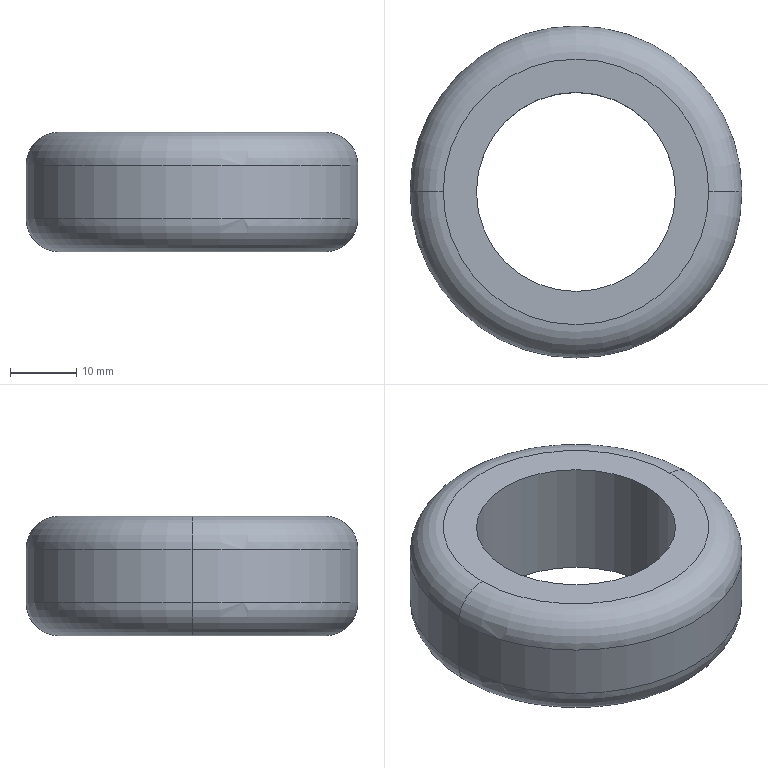Part | SolidWorks | features BaseBody 1 | 1 solid | 10 faces | box 50 x 50 x 18 mm | volume 21009 mm3 | torus 4 | cylinder 4 | plane 2 | commonest cylinder face diameters 30 x2 50 x2
STEP:
#1=CARTESIAN_POINT('',(-25.,0.,-13.));
#2=VERTEX_POINT('',#1);
#3=CARTESIAN_POINT('',(25.,0.,-13.));
#4=VERTEX_POINT('',#3);
#5=CARTESIAN_POINT('',(0.,0.,-13.));
#6=DIRECTION('',(0.,0.,-1.));
#7=DIRECTION('',(-1.,0.,0.));
#8=AXIS2_PLACEMENT_3D('',#5,#6,#7);
#9=CIRCLE('',#8,25.);
#10=EDGE_CURVE('',#2,#4,#9,.T.);
#11=ORIENTED_EDGE('',*,*,#10,.T.);
#12=CARTESIAN_POINT('',(20.,0.,-18.));
#13=VERTEX_POINT('',#12);
#14=CARTESIAN_POINT('',(20.,0.,-13.));
#15=DIRECTION('',(0.,1.,0.));
#16=DIRECTION('',(-1.,0.,0.));
#17=AXIS2_PLACEMENT_3D('',#14,#15,#16);
#18=CIRCLE('',#17,5.);
#19=EDGE_CURVE('',#4,#13,#18,.T.);
#20=ORIENTED_EDGE('',*,*,#19,.T.);
#21=CARTESIAN_POINT('',(-20.,0.,-18.));
#22=VERTEX_POINT('',#21);
#23=CARTESIAN_POINT('',(0.,0.,-18.));
#24=DIRECTION('',(0.,0.,1.));
#25=DIRECTION('',(-1.,0.,0.));
#26=AXIS2_PLACEMENT_3D('',#23,#24,#25);
#27=CIRCLE('',#26,20.);
#28=EDGE_CURVE('',#13,#22,#27,.T.);
#29=ORIENTED_EDGE('',*,*,#28,.T.);
#30=CARTESIAN_POINT('',(-20.,0.,-13.));
#31=DIRECTION('',(0.,-1.,0.));
#32=DIRECTION('',(0.,0.,-1.));
#33=AXIS2_PLACEMENT_3D('',#30,#31,#32);
#34=CIRCLE('',#33,5.);
#35=EDGE_CURVE('',#2,#22,#34,.T.);
#36=ORIENTED_EDGE('',*,*,#35,.F.);
#37=EDGE_LOOP('',(#11,#20,#29,#36));
#38=FACE_OUTER_BOUND('',#37,.T.);
#39=CARTESIAN_POINT('',(0.,0.,-13.));
#40=DIRECTION('',(0.,0.,-1.));
#41=DIRECTION('',(-1.,0.,0.));
#42=AXIS2_PLACEMENT_3D('',#39,#40,#41);
#43=TOROIDAL_SURFACE('',#42,20.,5.);
#44=ADVANCED_FACE('',(#38),#43,.T.);
#45=CARTESIAN_POINT('',(0.,0.,-13.));
#46=DIRECTION('',(0.,0.,-1.));
#47=DIRECTION('',(-1.,0.,0.));
#48=AXIS2_PLACEMENT_3D('',#45,#46,#47);
#49=CIRCLE('',#48,25.);
#50=EDGE_CURVE('',#4,#2,#49,.T.);
#51=ORIENTED_EDGE('',*,*,#50,.F.);
#52=CARTESIAN_POINT('',(25.,0.,-5.));
#53=VERTEX_POINT('',#52);
#54=CARTESIAN_POINT('',(25.,0.,0.));
#55=DIRECTION('',(0.,0.,1.));
#56=VECTOR('',#55,1000.);
#57=LINE('',#54,#56);
#58=EDGE_CURVE('',#4,#53,#57,.T.);
#59=ORIENTED_EDGE('',*,*,#58,.T.);
#60=CARTESIAN_POINT('',(-25.,0.,-5.));
#61=VERTEX_POINT('',#60);
#62=CARTESIAN_POINT('',(0.,0.,-5.));
#63=DIRECTION('',(0.,0.,1.));
#64=DIRECTION('',(-1.,0.,0.));
#65=AXIS2_PLACEMENT_3D('',#62,#63,#64);
#66=CIRCLE('',#65,25.);
#67=EDGE_CURVE('',#61,#53,#66,.T.);
#68=ORIENTED_EDGE('',*,*,#67,.F.);
#69=CARTESIAN_POINT('',(-25.,0.,0.));
#70=DIRECTION('',(0.,0.,1.));
#71=VECTOR('',#70,1000.);
#72=LINE('',#69,#71);
#73=EDGE_CURVE('',#2,#61,#72,.T.);
#74=ORIENTED_EDGE('',*,*,#73,.F.);
#75=EDGE_LOOP('',(#51,#59,#68,#74));
#76=FACE_OUTER_BOUND('',#75,.T.);
#77=CARTESIAN_POINT('',(0.,0.,0.));
#78=DIRECTION('',(0.,0.,1.));
#79=DIRECTION('',(-1.,0.,0.));
#80=AXIS2_PLACEMENT_3D('',#77,#78,#79);
#81=CYLINDRICAL_SURFACE('',#80,25.);
#82=ADVANCED_FACE('',(#76),#81,.T.);
#83=CARTESIAN_POINT('',(-20.,0.,0.));
#84=VERTEX_POINT('',#83);
#85=CARTESIAN_POINT('',(20.,0.,0.));
#86=VERTEX_POINT('',#85);
#87=CARTESIAN_POINT('',(0.,0.,0.));
#88=DIRECTION('',(0.,0.,-1.));
#89=DIRECTION('',(-1.,0.,0.));
#90=AXIS2_PLACEMENT_3D('',#87,#88,#89);
#91=CIRCLE('',#90,20.);
#92=EDGE_CURVE('',#84,#86,#91,.T.);
#93=ORIENTED_EDGE('',*,*,#92,.T.);
#94=CARTESIAN_POINT('',(20.,0.,-5.));
#95=DIRECTION('',(0.,1.,0.));
#96=DIRECTION('',(-1.,0.,0.));
#97=AXIS2_PLACEMENT_3D('',#94,#95,#96);
#98=CIRCLE('',#97,5.);
#99=EDGE_CURVE('',#86,#53,#98,.T.);
#100=ORIENTED_EDGE('',*,*,#99,.T.);
#101=CARTESIAN_POINT('',(0.,0.,-5.));
#102=DIRECTION('',(0.,0.,1.));
#103=DIRECTION('',(-1.,0.,0.));
#104=AXIS2_PLACEMENT_3D('',#101,#102,#103);
#105=CIRCLE('',#104,25.);
#106=EDGE_CURVE('',#53,#61,#105,.T.);
#107=ORIENTED_EDGE('',*,*,#106,.T.);
#108=CARTESIAN_POINT('',(-20.,0.,-5.));
#109=DIRECTION('',(0.,-1.,0.));
#110=DIRECTION('',(0.,0.,-1.));
#111=AXIS2_PLACEMENT_3D('',#108,#109,#110);
#112=CIRCLE('',#111,5.);
#113=EDGE_CURVE('',#84,#61,#112,.T.);
#114=ORIENTED_EDGE('',*,*,#113,.F.);
#115=EDGE_LOOP('',(#93,#100,#107,#114));
#116=FACE_OUTER_BOUND('',#115,.T.);
#117=CARTESIAN_POINT('',(0.,0.,-5.));
#118=DIRECTION('',(0.,0.,-1.));
#119=DIRECTION('',(-1.,0.,0.));
#120=AXIS2_PLACEMENT_3D('',#117,#118,#119);
#121=TOROIDAL_SURFACE('',#120,20.,5.);
#122=ADVANCED_FACE('',(#116),#121,.T.);
#123=CARTESIAN_POINT('',(15.,0.,-18.));
#124=VERTEX_POINT('',#123);
#125=CARTESIAN_POINT('',(-15.,0.,-18.));
#126=VERTEX_POINT('',#125);
#127=CARTESIAN_POINT('',(0.,0.,-18.));
#128=DIRECTION('',(0.,0.,1.));
#129=DIRECTION('',(-1.,0.,0.));
#130=AXIS2_PLACEMENT_3D('',#127,#128,#129);
#131=CIRCLE('',#130,15.);
#132=EDGE_CURVE('',#124,#126,#131,.T.);
#133=ORIENTED_EDGE('',*,*,#132,.F.);
#134=CARTESIAN_POINT('',(15.,0.,0.));
#135=VERTEX_POINT('',#134);
#136=CARTESIAN_POINT('',(15.,0.,0.));
#137=DIRECTION('',(0.,0.,1.));
#138=VECTOR('',#137,1000.);
#139=LINE('',#136,#138);
#140=EDGE_CURVE('',#124,#135,#139,.T.);
#141=ORIENTED_EDGE('',*,*,#140,.T.);
#142=CARTESIAN_POINT('',(-15.,0.,0.));
#143=VERTEX_POINT('',#142);
#144=CARTESIAN_POINT('',(0.,0.,0.));
#145=DIRECTION('',(0.,0.,-1.));
#146=DIRECTION('',(-1.,0.,0.));
#147=AXIS2_PLACEMENT_3D('',#144,#145,#146);
#148=CIRCLE('',#147,15.);
#149=EDGE_CURVE('',#143,#135,#148,.T.);
#150=ORIENTED_EDGE('',*,*,#149,.F.);
#151=CARTESIAN_POINT('',(-15.,0.,0.));
#152=DIRECTION('',(0.,0.,1.));
#153=VECTOR('',#152,1000.);
#154=LINE('',#151,#153);
#155=EDGE_CURVE('',#126,#143,#154,.T.);
#156=ORIENTED_EDGE('',*,*,#155,.F.);
#157=EDGE_LOOP('',(#133,#141,#150,#156));
#158=FACE_OUTER_BOUND('',#157,.T.);
#159=CARTESIAN_POINT('',(0.,0.,0.));
#160=DIRECTION('',(0.,0.,1.));
#161=DIRECTION('',(-1.,0.,0.));
#162=AXIS2_PLACEMENT_3D('',#159,#160,#161);
#163=CYLINDRICAL_SURFACE('',#162,15.);
#164=ADVANCED_FACE('',(#158),#163,.F.);
#165=CARTESIAN_POINT('',(0.,0.,-18.));
#166=DIRECTION('',(0.,0.,1.));
#167=DIRECTION('',(-1.,0.,0.));
#168=AXIS2_PLACEMENT_3D('',#165,#166,#167);
#169=CIRCLE('',#168,15.);
#170=EDGE_CURVE('',#126,#124,#169,.T.);
#171=ORIENTED_EDGE('',*,*,#170,.T.);
#172=ORIENTED_EDGE('',*,*,#132,.T.);
#173=EDGE_LOOP('',(#171,#172));
#174=FACE_BOUND('',#173,.T.);
#175=CARTESIAN_POINT('',(0.,0.,-18.));
#176=DIRECTION('',(0.,0.,1.));
#177=DIRECTION('',(-1.,0.,0.));
#178=AXIS2_PLACEMENT_3D('',#175,#176,#177);
#179=CIRCLE('',#178,20.);
#180=EDGE_CURVE('',#22,#13,#179,.T.);
#181=ORIENTED_EDGE('',*,*,#180,.F.);
#182=ORIENTED_EDGE('',*,*,#28,.F.);
#183=EDGE_LOOP('',(#181,#182));
#184=FACE_OUTER_BOUND('',#183,.T.);
#185=CARTESIAN_POINT('',(0.,0.,-18.));
#186=DIRECTION('',(0.,0.,1.));
#187=DIRECTION('',(1.,0.,0.));
#188=AXIS2_PLACEMENT_3D('',#185,#186,#187);
#189=PLANE('',#188);
#190=ADVANCED_FACE('',(#174,#184),#189,.F.);
#191=ORIENTED_EDGE('',*,*,#149,.T.);
#192=CARTESIAN_POINT('',(0.,0.,0.));
#193=DIRECTION('',(0.,0.,-1.));
#194=DIRECTION('',(-1.,0.,0.));
#195=AXIS2_PLACEMENT_3D('',#192,#193,#194);
#196=CIRCLE('',#195,15.);
#197=EDGE_CURVE('',#135,#143,#196,.T.);
#198=ORIENTED_EDGE('',*,*,#197,.T.);
#199=EDGE_LOOP('',(#191,#198));
#200=FACE_BOUND('',#199,.T.);
#201=ORIENTED_EDGE('',*,*,#92,.F.);
#202=CARTESIAN_POINT('',(0.,0.,0.));
#203=DIRECTION('',(0.,0.,-1.));
#204=DIRECTION('',(-1.,0.,0.));
#205=AXIS2_PLACEMENT_3D('',#202,#203,#204);
#206=CIRCLE('',#205,20.);
#207=EDGE_CURVE('',#86,#84,#206,.T.);
#208=ORIENTED_EDGE('',*,*,#207,.F.);
#209=EDGE_LOOP('',(#201,#208));
#210=FACE_OUTER_BOUND('',#209,.T.);
#211=CARTESIAN_POINT('',(0.,0.,0.));
#212=DIRECTION('',(0.,0.,1.));
#213=DIRECTION('',(1.,0.,0.));
#214=AXIS2_PLACEMENT_3D('',#211,#212,#213);
#215=PLANE('',#214);
#216=ADVANCED_FACE('',(#200,#210),#215,.T.);
#217=ORIENTED_EDGE('',*,*,#140,.F.);
#218=ORIENTED_EDGE('',*,*,#170,.F.);
#219=ORIENTED_EDGE('',*,*,#155,.T.);
#220=ORIENTED_EDGE('',*,*,#197,.F.);
#221=EDGE_LOOP('',(#217,#218,#219,#220));
#222=FACE_OUTER_BOUND('',#221,.T.);
#223=CARTESIAN_POINT('',(0.,0.,0.));
#224=DIRECTION('',(0.,0.,1.));
#225=DIRECTION('',(-1.,0.,0.));
#226=AXIS2_PLACEMENT_3D('',#223,#224,#225);
#227=CYLINDRICAL_SURFACE('',#226,15.);
#228=ADVANCED_FACE('',(#222),#227,.F.);
#229=ORIENTED_EDGE('',*,*,#99,.F.);
#230=ORIENTED_EDGE('',*,*,#207,.T.);
#231=ORIENTED_EDGE('',*,*,#113,.T.);
#232=ORIENTED_EDGE('',*,*,#67,.T.);
#233=EDGE_LOOP('',(#229,#230,#231,#232));
#234=FACE_OUTER_BOUND('',#233,.T.);
#235=CARTESIAN_POINT('',(0.,0.,-5.));
#236=DIRECTION('',(0.,0.,-1.));
#237=DIRECTION('',(-1.,0.,0.));
#238=AXIS2_PLACEMENT_3D('',#235,#236,#237);
#239=TOROIDAL_SURFACE('',#238,20.,5.);
#240=ADVANCED_FACE('',(#234),#239,.T.);
#241=ORIENTED_EDGE('',*,*,#58,.F.);
#242=ORIENTED_EDGE('',*,*,#10,.F.);
#243=ORIENTED_EDGE('',*,*,#73,.T.);
#244=ORIENTED_EDGE('',*,*,#106,.F.);
#245=EDGE_LOOP('',(#241,#242,#243,#244));
#246=FACE_OUTER_BOUND('',#245,.T.);
#247=CARTESIAN_POINT('',(0.,0.,0.));
#248=DIRECTION('',(0.,0.,1.));
#249=DIRECTION('',(-1.,0.,0.));
#250=AXIS2_PLACEMENT_3D('',#247,#248,#249);
#251=CYLINDRICAL_SURFACE('',#250,25.);
#252=ADVANCED_FACE('',(#246),#251,.T.);
#253=ORIENTED_EDGE('',*,*,#19,.F.);
#254=ORIENTED_EDGE('',*,*,#50,.T.);
#255=ORIENTED_EDGE('',*,*,#35,.T.);
#256=ORIENTED_EDGE('',*,*,#180,.T.);
#257=EDGE_LOOP('',(#253,#254,#255,#256));
#258=FACE_OUTER_BOUND('',#257,.T.);
#259=CARTESIAN_POINT('',(0.,0.,-13.));
#260=DIRECTION('',(0.,0.,-1.));
#261=DIRECTION('',(-1.,0.,0.));
#262=AXIS2_PLACEMENT_3D('',#259,#260,#261);
#263=TOROIDAL_SURFACE('',#262,20.,5.);
#264=ADVANCED_FACE('',(#258),#263,.T.);
#265=CLOSED_SHELL('',(#44,#82,#122,#164,#190,#216,#228,#240,#252,#264));
#266=MANIFOLD_SOLID_BREP('',#265);
#267=CARTESIAN_POINT('',(0.,0.,0.));
#268=DIRECTION('',(0.,0.,1.));
#269=DIRECTION('',(1.,0.,0.));
#270=AXIS2_PLACEMENT_3D('',#267,#268,#269);
#271=(LENGTH_UNIT()NAMED_UNIT(*)SI_UNIT(.MILLI.,.METRE.));
#272=UNCERTAINTY_MEASURE_WITH_UNIT(LENGTH_MEASURE(0.00001),#271,'','');
#273=(NAMED_UNIT(*)PLANE_ANGLE_UNIT()SI_UNIT($,.RADIAN.));
#274=(NAMED_UNIT(*)SI_UNIT($,.STERADIAN.)SOLID_ANGLE_UNIT());
#275=(GEOMETRIC_REPRESENTATION_CONTEXT(3)GLOBAL_UNCERTAINTY_ASSIGNED_CONTEXT((#272))GLOBAL_UNIT_ASSIGNED_CONTEXT((#271,#273,#274))REPRESENTATION_CONTEXT('',''));
#276=ADVANCED_BREP_SHAPE_REPRESENTATION('',(#266,#270),#275);